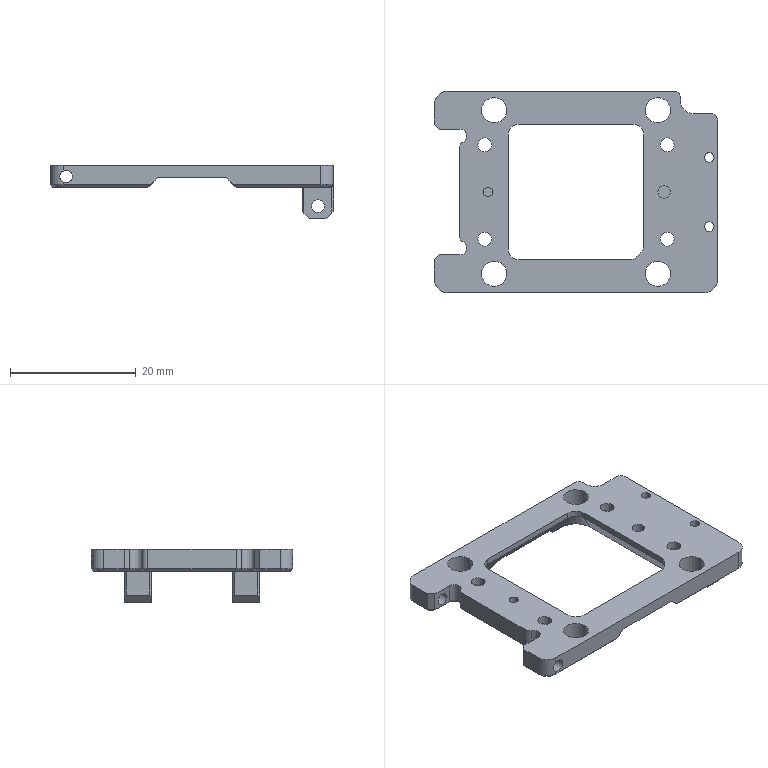NC program | NX | posted with a generic post | part box 45 x 32 x 8.5 mm
Whole program:
N10 G17 G21 G94 G90
(DRILLING_COPY_COPY_2 , TOOL : D4A45)
N12 T14 M6
N14 G54
N16 G17 G0 G90 X20. Y-6.5 B0. C0. S5000 M3
N18 G43 Z30. H14
N20 G94 G81 G98 Z-6.35 F250. R-2.25
N22 X-20. Y-1.8 Z-1.1 R3.
N24 G80
N26 G0 X-20. Y-1.8 Z30.
N28 M5
(DRILLING_COPY_COPY_COPY_1_COPY , TOOL : 2.02ZT)
N30 T18 M6
N32 G54
N34 G17 G0 G90 X-20. Y-1.8 B0. C0. S1447 M3
N36 G43 Z30. H18
N38 G94 G83 G98 Z-8.107 F100. Q2. R3.
N40 X20. Y-6.5 Z-11.607 R-2.25
N42 G80
N44 G0 X20. Y-6.5 Z30.
N46 M5
N48 M2